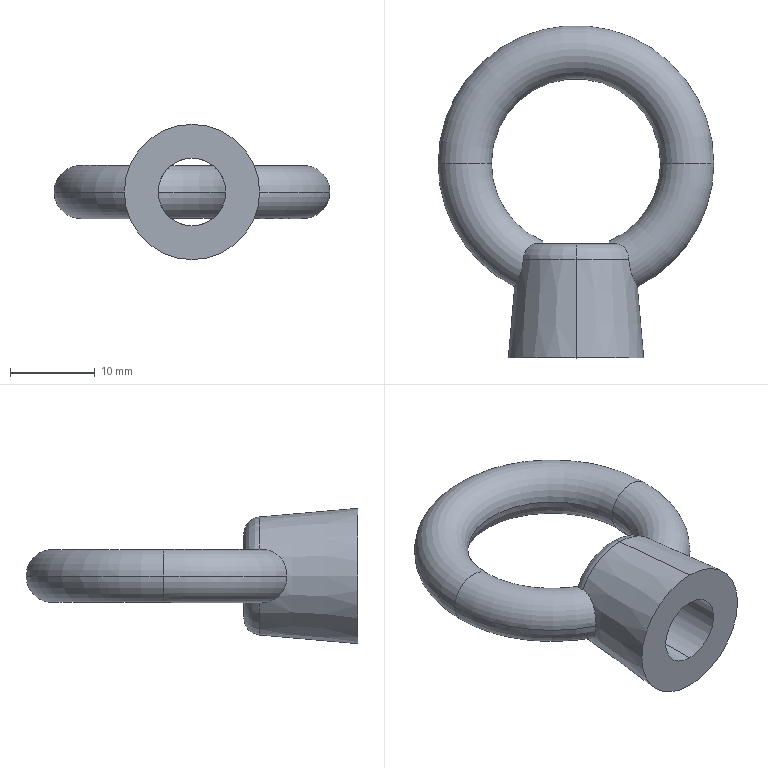Part | STEP file | B-1132-8 | 1 solid | 16 faces | box 32.6 x 39.3 x 16 mm | volume 3782 mm3 | torus 9 | plane 3 | cylinder 2 | cone 2 | commonest cylinder face diameters 8 x2
STEP:
#1=CARTESIAN_POINT('',(16.3,0.,0.));
#2=VERTEX_POINT('',#1);
#3=CARTESIAN_POINT('',(10.,0.,0.));
#4=VERTEX_POINT('',#3);
#5=CARTESIAN_POINT('',(13.15,0.,0.));
#6=DIRECTION('',(0.,1.,0.));
#7=DIRECTION('',(-1.,0.,0.));
#8=AXIS2_PLACEMENT_3D('',#5,#6,#7);
#9=CIRCLE('',#8,3.15);
#10=EDGE_CURVE('',#2,#4,#9,.T.);
#11=ORIENTED_EDGE('',*,*,#10,.F.);
#12=CARTESIAN_POINT('',(7.264,-14.592,0.));
#13=VERTEX_POINT('',#12);
#14=CARTESIAN_POINT('',(0.,0.,0.));
#15=DIRECTION('',(0.,0.,-1.));
#16=DIRECTION('',(-1.,0.,0.));
#17=AXIS2_PLACEMENT_3D('',#14,#15,#16);
#18=CIRCLE('',#17,16.3);
#19=EDGE_CURVE('',#2,#13,#18,.T.);
#20=ORIENTED_EDGE('',*,*,#19,.T.);
#21=CARTESIAN_POINT('',(6.231,-11.326,-3.142));
#22=VERTEX_POINT('',#21);
#23=CARTESIAN_POINT('',(7.264,-14.592,0.));
#24=CARTESIAN_POINT('',(7.264,-14.592,-0.2184));
#25=CARTESIAN_POINT('',(7.253,-14.572,-0.4352));
#26=CARTESIAN_POINT('',(7.207,-14.494,-0.8657));
#27=CARTESIAN_POINT('',(7.173,-14.435,-1.075));
#28=CARTESIAN_POINT('',(7.088,-14.28,-1.474));
#29=CARTESIAN_POINT('',(7.036,-14.183,-1.666));
#30=CARTESIAN_POINT('',(6.922,-13.953,-2.022));
#31=CARTESIAN_POINT('',(6.859,-13.822,-2.184));
#32=CARTESIAN_POINT('',(6.731,-13.524,-2.478));
#33=CARTESIAN_POINT('',(6.665,-13.357,-2.61));
#34=CARTESIAN_POINT('',(6.541,-13.001,-2.828));
#35=CARTESIAN_POINT('',(6.483,-12.81,-2.918));
#36=CARTESIAN_POINT('',(6.38,-12.403,-3.055));
#37=CARTESIAN_POINT('',(6.337,-12.194,-3.101));
#38=CARTESIAN_POINT('',(6.27,-11.765,-3.152));
#39=CARTESIAN_POINT('',(6.246,-11.544,-3.156));
#40=CARTESIAN_POINT('',(6.231,-11.326,-3.142));
#41=B_SPLINE_CURVE_WITH_KNOTS('',3,(#23,#24,#25,#26,#27,#28,#29,#30,#31,#32,#33,#34,#35,#36,#37,#38,#39,#40),.UNSPECIFIED.,.F.,.F.,(4,2,2,2,2,2,2,2,4),(0.007106,0.007756,0.008406,0.009056,0.009706,0.01036,0.01101,0.01166,0.01231),.UNSPECIFIED.);
#42=EDGE_CURVE('',#13,#22,#41,.T.);
#43=ORIENTED_EDGE('',*,*,#42,.T.);
#44=CARTESIAN_POINT('',(4.645,-9.5,-1.814));
#45=VERTEX_POINT('',#44);
#46=CARTESIAN_POINT('',(6.231,-11.326,-3.142));
#47=CARTESIAN_POINT('',(6.223,-11.199,-3.134));
#48=CARTESIAN_POINT('',(6.205,-11.075,-3.119));
#49=CARTESIAN_POINT('',(6.15,-10.834,-3.075));
#50=CARTESIAN_POINT('',(6.113,-10.715,-3.046));
#51=CARTESIAN_POINT('',(6.024,-10.49,-2.971));
#52=CARTESIAN_POINT('',(5.972,-10.385,-2.927));
#53=CARTESIAN_POINT('',(5.855,-10.187,-2.824));
#54=CARTESIAN_POINT('',(5.788,-10.095,-2.765));
#55=CARTESIAN_POINT('',(5.575,-9.848,-2.574));
#56=CARTESIAN_POINT('',(5.411,-9.719,-2.422));
#57=CARTESIAN_POINT('',(5.055,-9.547,-2.112));
#58=CARTESIAN_POINT('',(4.861,-9.5,-1.949));
#59=CARTESIAN_POINT('',(4.645,-9.5,-1.814));
#60=B_SPLINE_CURVE_WITH_KNOTS('',3,(#46,#47,#48,#49,#50,#51,#52,#53,#54,#55,#56,#57,#58,#59),.UNSPECIFIED.,.F.,.F.,(4,2,2,2,2,2,4),(0.,0.0003768,0.0007536,0.00113,0.001507,0.002261,0.003014),.UNSPECIFIED.);
#61=EDGE_CURVE('',#22,#45,#60,.T.);
#62=ORIENTED_EDGE('',*,*,#61,.T.);
#63=CARTESIAN_POINT('',(3.816,-9.5,-1.2));
#64=VERTEX_POINT('',#63);
#65=CARTESIAN_POINT('',(4.645,-9.5,-1.814));
#66=CARTESIAN_POINT('',(4.5,-9.5,-1.723));
#67=CARTESIAN_POINT('',(4.357,-9.5,-1.628));
#68=CARTESIAN_POINT('',(4.08,-9.5,-1.425));
#69=CARTESIAN_POINT('',(3.944,-9.5,-1.316));
#70=CARTESIAN_POINT('',(3.816,-9.5,-1.2));
#71=B_SPLINE_CURVE_WITH_KNOTS('',3,(#65,#66,#67,#68,#69,#70),.UNSPECIFIED.,.F.,.F.,(4,2,4),(0.02444,0.02495,0.02546),.UNSPECIFIED.);
#72=EDGE_CURVE('',#45,#64,#71,.T.);
#73=ORIENTED_EDGE('',*,*,#72,.T.);
#74=CARTESIAN_POINT('',(4.,-9.165,0.));
#75=VERTEX_POINT('',#74);
#76=CARTESIAN_POINT('',(3.816,-9.5,-1.2));
#77=CARTESIAN_POINT('',(3.872,-9.398,-1.021));
#78=CARTESIAN_POINT('',(3.918,-9.314,-0.8311));
#79=CARTESIAN_POINT('',(3.983,-9.196,-0.4221));
#80=CARTESIAN_POINT('',(4.,-9.165,-0.2133));
#81=CARTESIAN_POINT('',(4.,-9.165,0.));
#82=B_SPLINE_CURVE_WITH_KNOTS('',3,(#76,#77,#78,#79,#80,#81),.UNSPECIFIED.,.F.,.F.,(4,2,4),(0.00665,0.007285,0.00792),.UNSPECIFIED.);
#83=EDGE_CURVE('',#64,#75,#82,.T.);
#84=ORIENTED_EDGE('',*,*,#83,.T.);
#85=CARTESIAN_POINT('',(0.,0.,0.));
#86=DIRECTION('',(0.,0.,-1.));
#87=DIRECTION('',(-1.,0.,0.));
#88=AXIS2_PLACEMENT_3D('',#85,#86,#87);
#89=CIRCLE('',#88,10.);
#90=EDGE_CURVE('',#4,#75,#89,.T.);
#91=ORIENTED_EDGE('',*,*,#90,.F.);
#92=EDGE_LOOP('',(#11,#20,#43,#62,#73,#84,#91));
#93=FACE_OUTER_BOUND('',#92,.T.);
#94=CARTESIAN_POINT('',(0.,0.,0.));
#95=DIRECTION('',(0.,0.,-1.));
#96=DIRECTION('',(-1.,0.,0.));
#97=AXIS2_PLACEMENT_3D('',#94,#95,#96);
#98=TOROIDAL_SURFACE('',#97,13.15,3.15);
#99=ADVANCED_FACE('',(#93),#98,.T.);
#100=CARTESIAN_POINT('',(-6.231,-11.326,-3.142));
#101=VERTEX_POINT('',#100);
#102=CARTESIAN_POINT('',(-7.264,-14.592,0.));
#103=VERTEX_POINT('',#102);
#104=CARTESIAN_POINT('',(-6.231,-11.326,-3.142));
#105=CARTESIAN_POINT('',(-6.246,-11.543,-3.156));
#106=CARTESIAN_POINT('',(-6.269,-11.76,-3.152));
#107=CARTESIAN_POINT('',(-6.336,-12.191,-3.101));
#108=CARTESIAN_POINT('',(-6.38,-12.403,-3.055));
#109=CARTESIAN_POINT('',(-6.481,-12.804,-2.92));
#110=CARTESIAN_POINT('',(-6.54,-12.997,-2.831));
#111=CARTESIAN_POINT('',(-6.665,-13.357,-2.61));
#112=CARTESIAN_POINT('',(-6.729,-13.52,-2.482));
#113=CARTESIAN_POINT('',(-6.858,-13.819,-2.188));
#114=CARTESIAN_POINT('',(-6.922,-13.953,-2.022));
#115=CARTESIAN_POINT('',(-7.036,-14.181,-1.668));
#116=CARTESIAN_POINT('',(-7.087,-14.278,-1.478));
#117=CARTESIAN_POINT('',(-7.174,-14.435,-1.075));
#118=CARTESIAN_POINT('',(-7.207,-14.493,-0.8672));
#119=CARTESIAN_POINT('',(-7.252,-14.572,-0.4401));
#120=CARTESIAN_POINT('',(-7.264,-14.592,-0.2184));
#121=CARTESIAN_POINT('',(-7.264,-14.592,0.));
#122=B_SPLINE_CURVE_WITH_KNOTS('',3,(#104,#105,#106,#107,#108,#109,#110,#111,#112,#113,#114,#115,#116,#117,#118,#119,#120,#121),.UNSPECIFIED.,.F.,.F.,(4,2,2,2,2,2,2,2,4),(0.001904,0.002554,0.003205,0.003855,0.004505,0.005155,0.005805,0.006456,0.007106),.UNSPECIFIED.);
#123=EDGE_CURVE('',#101,#103,#122,.T.);
#124=ORIENTED_EDGE('',*,*,#123,.T.);
#125=CARTESIAN_POINT('',(-16.3,0.,0.));
#126=VERTEX_POINT('',#125);
#127=CARTESIAN_POINT('',(0.,0.,0.));
#128=DIRECTION('',(0.,0.,-1.));
#129=DIRECTION('',(-1.,0.,0.));
#130=AXIS2_PLACEMENT_3D('',#127,#128,#129);
#131=CIRCLE('',#130,16.3);
#132=EDGE_CURVE('',#103,#126,#131,.T.);
#133=ORIENTED_EDGE('',*,*,#132,.T.);
#134=CARTESIAN_POINT('',(-10.,0.,0.));
#135=VERTEX_POINT('',#134);
#136=CARTESIAN_POINT('',(-13.15,0.,0.));
#137=DIRECTION('',(0.,-1.,0.));
#138=DIRECTION('',(0.,0.,-1.));
#139=AXIS2_PLACEMENT_3D('',#136,#137,#138);
#140=CIRCLE('',#139,3.15);
#141=EDGE_CURVE('',#126,#135,#140,.T.);
#142=ORIENTED_EDGE('',*,*,#141,.T.);
#143=CARTESIAN_POINT('',(-4.,-9.165,0.));
#144=VERTEX_POINT('',#143);
#145=CARTESIAN_POINT('',(0.,0.,0.));
#146=DIRECTION('',(0.,0.,-1.));
#147=DIRECTION('',(-1.,0.,0.));
#148=AXIS2_PLACEMENT_3D('',#145,#146,#147);
#149=CIRCLE('',#148,10.);
#150=EDGE_CURVE('',#144,#135,#149,.T.);
#151=ORIENTED_EDGE('',*,*,#150,.F.);
#152=CARTESIAN_POINT('',(-3.816,-9.5,-1.2));
#153=VERTEX_POINT('',#152);
#154=CARTESIAN_POINT('',(-4.,-9.165,0.));
#155=CARTESIAN_POINT('',(-4.,-9.165,-0.1064));
#156=CARTESIAN_POINT('',(-3.996,-9.173,-0.2143));
#157=CARTESIAN_POINT('',(-3.979,-9.204,-0.4241));
#158=CARTESIAN_POINT('',(-3.966,-9.226,-0.527));
#159=CARTESIAN_POINT('',(-3.918,-9.314,-0.8302));
#160=CARTESIAN_POINT('',(-3.871,-9.399,-1.023));
#161=CARTESIAN_POINT('',(-3.816,-9.5,-1.2));
#162=B_SPLINE_CURVE_WITH_KNOTS('',3,(#154,#155,#156,#157,#158,#159,#160,#161),.UNSPECIFIED.,.F.,.F.,(4,2,2,4),(0.00792,0.008237,0.008554,0.009188),.UNSPECIFIED.);
#163=EDGE_CURVE('',#144,#153,#162,.T.);
#164=ORIENTED_EDGE('',*,*,#163,.T.);
#165=CARTESIAN_POINT('',(-4.645,-9.5,-1.814));
#166=VERTEX_POINT('',#165);
#167=CARTESIAN_POINT('',(-3.816,-9.5,-1.2));
#168=CARTESIAN_POINT('',(-3.943,-9.5,-1.316));
#169=CARTESIAN_POINT('',(-4.079,-9.5,-1.424));
#170=CARTESIAN_POINT('',(-4.357,-9.5,-1.628));
#171=CARTESIAN_POINT('',(-4.499,-9.5,-1.723));
#172=CARTESIAN_POINT('',(-4.645,-9.5,-1.814));
#173=B_SPLINE_CURVE_WITH_KNOTS('',3,(#167,#168,#169,#170,#171,#172),.UNSPECIFIED.,.F.,.F.,(4,2,4),(0.0236,0.02411,0.02462),.UNSPECIFIED.);
#174=EDGE_CURVE('',#153,#166,#173,.T.);
#175=ORIENTED_EDGE('',*,*,#174,.T.);
#176=CARTESIAN_POINT('',(-4.645,-9.5,-1.814));
#177=CARTESIAN_POINT('',(-4.753,-9.5,-1.881));
#178=CARTESIAN_POINT('',(-4.854,-9.512,-1.955));
#179=CARTESIAN_POINT('',(-5.049,-9.556,-2.108));
#180=CARTESIAN_POINT('',(-5.143,-9.589,-2.188));
#181=CARTESIAN_POINT('',(-5.322,-9.676,-2.344));
#182=CARTESIAN_POINT('',(-5.407,-9.729,-2.42));
#183=CARTESIAN_POINT('',(-5.568,-9.856,-2.567));
#184=CARTESIAN_POINT('',(-5.646,-9.93,-2.637));
#185=CARTESIAN_POINT('',(-5.788,-10.094,-2.765));
#186=CARTESIAN_POINT('',(-5.853,-10.185,-2.823));
#187=CARTESIAN_POINT('',(-5.971,-10.382,-2.926));
#188=CARTESIAN_POINT('',(-6.024,-10.49,-2.971));
#189=CARTESIAN_POINT('',(-6.157,-10.825,-3.082));
#190=CARTESIAN_POINT('',(-6.215,-11.072,-3.126));
#191=CARTESIAN_POINT('',(-6.231,-11.326,-3.142));
#192=B_SPLINE_CURVE_WITH_KNOTS('',3,(#176,#177,#178,#179,#180,#181,#182,#183,#184,#185,#186,#187,#188,#189,#190,#191),.UNSPECIFIED.,.F.,.F.,(4,2,2,2,2,2,2,4),(0.,0.0003768,0.0007535,0.00113,0.001507,0.001884,0.002261,0.003014),.UNSPECIFIED.);
#193=EDGE_CURVE('',#166,#101,#192,.T.);
#194=ORIENTED_EDGE('',*,*,#193,.T.);
#195=EDGE_LOOP('',(#124,#133,#142,#151,#164,#175,#194));
#196=FACE_OUTER_BOUND('',#195,.T.);
#197=CARTESIAN_POINT('',(0.,0.,0.));
#198=DIRECTION('',(0.,0.,-1.));
#199=DIRECTION('',(-1.,0.,0.));
#200=AXIS2_PLACEMENT_3D('',#197,#198,#199);
#201=TOROIDAL_SURFACE('',#200,13.15,3.15);
#202=ADVANCED_FACE('',(#196),#201,.T.);
#203=ORIENTED_EDGE('',*,*,#141,.F.);
#204=CARTESIAN_POINT('',(0.,0.,0.));
#205=DIRECTION('',(0.,0.,-1.));
#206=DIRECTION('',(-1.,0.,0.));
#207=AXIS2_PLACEMENT_3D('',#204,#205,#206);
#208=CIRCLE('',#207,16.3);
#209=EDGE_CURVE('',#126,#2,#208,.T.);
#210=ORIENTED_EDGE('',*,*,#209,.T.);
#211=ORIENTED_EDGE('',*,*,#10,.T.);
#212=CARTESIAN_POINT('',(0.,0.,0.));
#213=DIRECTION('',(0.,0.,-1.));
#214=DIRECTION('',(-1.,0.,0.));
#215=AXIS2_PLACEMENT_3D('',#212,#213,#214);
#216=CIRCLE('',#215,10.);
#217=EDGE_CURVE('',#135,#4,#216,.T.);
#218=ORIENTED_EDGE('',*,*,#217,.F.);
#219=EDGE_LOOP('',(#203,#210,#211,#218));
#220=FACE_OUTER_BOUND('',#219,.T.);
#221=CARTESIAN_POINT('',(0.,0.,0.));
#222=DIRECTION('',(0.,0.,-1.));
#223=DIRECTION('',(-1.,0.,0.));
#224=AXIS2_PLACEMENT_3D('',#221,#222,#223);
#225=TOROIDAL_SURFACE('',#224,13.15,3.15);
#226=ADVANCED_FACE('',(#220),#225,.T.);
#227=CARTESIAN_POINT('',(0.,-11.326,6.979));
#228=VERTEX_POINT('',#227);
#229=CARTESIAN_POINT('',(-6.231,-11.326,3.142));
#230=VERTEX_POINT('',#229);
#231=CARTESIAN_POINT('',(0.,-11.326,0.));
#232=DIRECTION('',(0.,-1.,0.));
#233=DIRECTION('',(0.,0.,1.));
#234=AXIS2_PLACEMENT_3D('',#231,#232,#233);
#235=CIRCLE('',#234,6.979);
#236=EDGE_CURVE('',#228,#230,#235,.T.);
#237=ORIENTED_EDGE('',*,*,#236,.F.);
#238=CARTESIAN_POINT('',(0.,-9.5,4.986));
#239=VERTEX_POINT('',#238);
#240=CARTESIAN_POINT('',(0.,-11.5,4.986));
#241=DIRECTION('',(-1.,0.,0.));
#242=DIRECTION('',(0.,0.,1.));
#243=AXIS2_PLACEMENT_3D('',#240,#241,#242);
#244=CIRCLE('',#243,2.);
#245=EDGE_CURVE('',#228,#239,#244,.T.);
#246=ORIENTED_EDGE('',*,*,#245,.T.);
#247=CARTESIAN_POINT('',(-4.645,-9.5,1.814));
#248=VERTEX_POINT('',#247);
#249=CARTESIAN_POINT('',(0.,-9.5,0.));
#250=DIRECTION('',(0.,1.,0.));
#251=DIRECTION('',(0.,0.,1.));
#252=AXIS2_PLACEMENT_3D('',#249,#250,#251);
#253=CIRCLE('',#252,4.986);
#254=EDGE_CURVE('',#248,#239,#253,.T.);
#255=ORIENTED_EDGE('',*,*,#254,.F.);
#256=CARTESIAN_POINT('',(-6.231,-11.326,3.142));
#257=CARTESIAN_POINT('',(-6.223,-11.199,3.134));
#258=CARTESIAN_POINT('',(-6.205,-11.075,3.119));
#259=CARTESIAN_POINT('',(-6.15,-10.834,3.075));
#260=CARTESIAN_POINT('',(-6.113,-10.715,3.046));
#261=CARTESIAN_POINT('',(-6.024,-10.49,2.971));
#262=CARTESIAN_POINT('',(-5.972,-10.385,2.927));
#263=CARTESIAN_POINT('',(-5.855,-10.187,2.824));
#264=CARTESIAN_POINT('',(-5.788,-10.095,2.765));
#265=CARTESIAN_POINT('',(-5.575,-9.848,2.574));
#266=CARTESIAN_POINT('',(-5.411,-9.719,2.422));
#267=CARTESIAN_POINT('',(-5.055,-9.547,2.112));
#268=CARTESIAN_POINT('',(-4.861,-9.5,1.949));
#269=CARTESIAN_POINT('',(-4.645,-9.5,1.814));
#270=B_SPLINE_CURVE_WITH_KNOTS('',3,(#256,#257,#258,#259,#260,#261,#262,#263,#264,#265,#266,#267,#268,#269),.UNSPECIFIED.,.F.,.F.,(4,2,2,2,2,2,4),(0.,0.0003768,0.0007536,0.00113,0.001507,0.002261,0.003014),.UNSPECIFIED.);
#271=EDGE_CURVE('',#230,#248,#270,.T.);
#272=ORIENTED_EDGE('',*,*,#271,.F.);
#273=EDGE_LOOP('',(#237,#246,#255,#272));
#274=FACE_OUTER_BOUND('',#273,.T.);
#275=CARTESIAN_POINT('',(0.,-11.5,0.));
#276=DIRECTION('',(0.,1.,0.));
#277=DIRECTION('',(0.,0.,1.));
#278=AXIS2_PLACEMENT_3D('',#275,#276,#277);
#279=TOROIDAL_SURFACE('',#278,4.986,2.);
#280=ADVANCED_FACE('',(#274),#279,.T.);
#281=CARTESIAN_POINT('',(-3.816,-9.5,1.2));
#282=VERTEX_POINT('',#281);
#283=CARTESIAN_POINT('',(0.,-9.5,4.));
#284=VERTEX_POINT('',#283);
#285=CARTESIAN_POINT('',(0.,-9.5,0.));
#286=DIRECTION('',(0.,1.,0.));
#287=DIRECTION('',(0.,0.,1.));
#288=AXIS2_PLACEMENT_3D('',#285,#286,#287);
#289=CIRCLE('',#288,4.);
#290=EDGE_CURVE('',#282,#284,#289,.T.);
#291=ORIENTED_EDGE('',*,*,#290,.T.);
#292=CARTESIAN_POINT('',(0.,-23.,4.));
#293=VERTEX_POINT('',#292);
#294=CARTESIAN_POINT('',(0.,-5.,4.));
#295=DIRECTION('',(0.,-1.,0.));
#296=VECTOR('',#295,1000.);
#297=LINE('',#294,#296);
#298=EDGE_CURVE('',#284,#293,#297,.T.);
#299=ORIENTED_EDGE('',*,*,#298,.T.);
#300=CARTESIAN_POINT('',(0.,-23.,-4.));
#301=VERTEX_POINT('',#300);
#302=CARTESIAN_POINT('',(0.,-23.,0.));
#303=DIRECTION('',(0.,-1.,0.));
#304=DIRECTION('',(0.,0.,-1.));
#305=AXIS2_PLACEMENT_3D('',#302,#303,#304);
#306=CIRCLE('',#305,4.);
#307=EDGE_CURVE('',#293,#301,#306,.T.);
#308=ORIENTED_EDGE('',*,*,#307,.T.);
#309=CARTESIAN_POINT('',(0.,-9.5,-4.));
#310=VERTEX_POINT('',#309);
#311=CARTESIAN_POINT('',(0.,-5.,-4.));
#312=DIRECTION('',(0.,-1.,0.));
#313=VECTOR('',#312,1000.);
#314=LINE('',#311,#313);
#315=EDGE_CURVE('',#310,#301,#314,.T.);
#316=ORIENTED_EDGE('',*,*,#315,.F.);
#317=CARTESIAN_POINT('',(0.,-9.5,0.));
#318=DIRECTION('',(0.,1.,0.));
#319=DIRECTION('',(0.,0.,1.));
#320=AXIS2_PLACEMENT_3D('',#317,#318,#319);
#321=CIRCLE('',#320,4.);
#322=EDGE_CURVE('',#310,#153,#321,.T.);
#323=ORIENTED_EDGE('',*,*,#322,.T.);
#324=ORIENTED_EDGE('',*,*,#163,.F.);
#325=CARTESIAN_POINT('',(-3.816,-9.5,1.2));
#326=CARTESIAN_POINT('',(-3.872,-9.398,1.021));
#327=CARTESIAN_POINT('',(-3.918,-9.314,0.8311));
#328=CARTESIAN_POINT('',(-3.983,-9.196,0.4221));
#329=CARTESIAN_POINT('',(-4.,-9.165,0.2133));
#330=CARTESIAN_POINT('',(-4.,-9.165,0.));
#331=B_SPLINE_CURVE_WITH_KNOTS('',3,(#325,#326,#327,#328,#329,#330),.UNSPECIFIED.,.F.,.F.,(4,2,4),(0.00665,0.007285,0.00792),.UNSPECIFIED.);
#332=EDGE_CURVE('',#282,#144,#331,.T.);
#333=ORIENTED_EDGE('',*,*,#332,.F.);
#334=EDGE_LOOP('',(#291,#299,#308,#316,#323,#324,#333));
#335=FACE_OUTER_BOUND('',#334,.T.);
#336=CARTESIAN_POINT('',(0.,-5.,0.));
#337=DIRECTION('',(0.,-1.,0.));
#338=DIRECTION('',(0.,0.,-1.));
#339=AXIS2_PLACEMENT_3D('',#336,#337,#338);
#340=CYLINDRICAL_SURFACE('',#339,4.);
#341=ADVANCED_FACE('',(#335),#340,.F.);
#342=ORIENTED_EDGE('',*,*,#209,.F.);
#343=CARTESIAN_POINT('',(-13.15,0.,0.));
#344=DIRECTION('',(0.,-1.,0.));
#345=DIRECTION('',(0.,0.,-1.));
#346=AXIS2_PLACEMENT_3D('',#343,#344,#345);
#347=CIRCLE('',#346,3.15);
#348=EDGE_CURVE('',#135,#126,#347,.T.);
#349=ORIENTED_EDGE('',*,*,#348,.F.);
#350=ORIENTED_EDGE('',*,*,#217,.T.);
#351=CARTESIAN_POINT('',(13.15,0.,0.));
#352=DIRECTION('',(0.,1.,0.));
#353=DIRECTION('',(-1.,0.,0.));
#354=AXIS2_PLACEMENT_3D('',#351,#352,#353);
#355=CIRCLE('',#354,3.15);
#356=EDGE_CURVE('',#4,#2,#355,.T.);
#357=ORIENTED_EDGE('',*,*,#356,.T.);
#358=EDGE_LOOP('',(#342,#349,#350,#357));
#359=FACE_OUTER_BOUND('',#358,.T.);
#360=CARTESIAN_POINT('',(0.,0.,0.));
#361=DIRECTION('',(0.,0.,-1.));
#362=DIRECTION('',(-1.,0.,0.));
#363=AXIS2_PLACEMENT_3D('',#360,#361,#362);
#364=TOROIDAL_SURFACE('',#363,13.15,3.15);
#365=ADVANCED_FACE('',(#359),#364,.T.);
#366=ORIENTED_EDGE('',*,*,#132,.F.);
#367=CARTESIAN_POINT('',(-7.264,-14.592,0.));
#368=CARTESIAN_POINT('',(-7.264,-14.592,0.2184));
#369=CARTESIAN_POINT('',(-7.253,-14.572,0.4352));
#370=CARTESIAN_POINT('',(-7.207,-14.494,0.8657));
#371=CARTESIAN_POINT('',(-7.173,-14.435,1.075));
#372=CARTESIAN_POINT('',(-7.088,-14.28,1.474));
#373=CARTESIAN_POINT('',(-7.036,-14.183,1.666));
#374=CARTESIAN_POINT('',(-6.922,-13.953,2.022));
#375=CARTESIAN_POINT('',(-6.859,-13.822,2.184));
#376=CARTESIAN_POINT('',(-6.731,-13.524,2.478));
#377=CARTESIAN_POINT('',(-6.665,-13.357,2.61));
#378=CARTESIAN_POINT('',(-6.541,-13.001,2.828));
#379=CARTESIAN_POINT('',(-6.483,-12.81,2.918));
#380=CARTESIAN_POINT('',(-6.38,-12.403,3.055));
#381=CARTESIAN_POINT('',(-6.337,-12.194,3.101));
#382=CARTESIAN_POINT('',(-6.27,-11.765,3.152));
#383=CARTESIAN_POINT('',(-6.246,-11.544,3.156));
#384=CARTESIAN_POINT('',(-6.231,-11.326,3.142));
#385=B_SPLINE_CURVE_WITH_KNOTS('',3,(#367,#368,#369,#370,#371,#372,#373,#374,#375,#376,#377,#378,#379,#380,#381,#382,#383,#384),.UNSPECIFIED.,.F.,.F.,(4,2,2,2,2,2,2,2,4),(0.007106,0.007756,0.008406,0.009056,0.009706,0.01036,0.01101,0.01166,0.01231),.UNSPECIFIED.);
#386=EDGE_CURVE('',#103,#230,#385,.T.);
#387=ORIENTED_EDGE('',*,*,#386,.T.);
#388=ORIENTED_EDGE('',*,*,#271,.T.);
#389=CARTESIAN_POINT('',(-4.645,-9.5,1.814));
#390=CARTESIAN_POINT('',(-4.5,-9.5,1.723));
#391=CARTESIAN_POINT('',(-4.357,-9.5,1.628));
#392=CARTESIAN_POINT('',(-4.08,-9.5,1.425));
#393=CARTESIAN_POINT('',(-3.944,-9.5,1.316));
#394=CARTESIAN_POINT('',(-3.816,-9.5,1.2));
#395=B_SPLINE_CURVE_WITH_KNOTS('',3,(#389,#390,#391,#392,#393,#394),.UNSPECIFIED.,.F.,.F.,(4,2,4),(0.01978,0.02029,0.0208),.UNSPECIFIED.);
#396=EDGE_CURVE('',#248,#282,#395,.T.);
#397=ORIENTED_EDGE('',*,*,#396,.T.);
#398=ORIENTED_EDGE('',*,*,#332,.T.);
#399=ORIENTED_EDGE('',*,*,#150,.T.);
#400=ORIENTED_EDGE('',*,*,#348,.T.);
#401=EDGE_LOOP('',(#366,#387,#388,#397,#398,#399,#400));
#402=FACE_OUTER_BOUND('',#401,.T.);
#403=CARTESIAN_POINT('',(0.,0.,0.));
#404=DIRECTION('',(0.,0.,-1.));
#405=DIRECTION('',(-1.,0.,0.));
#406=AXIS2_PLACEMENT_3D('',#403,#404,#405);
#407=TOROIDAL_SURFACE('',#406,13.15,3.15);
#408=ADVANCED_FACE('',(#402),#407,.T.);
#409=CARTESIAN_POINT('',(6.231,-11.326,3.142));
#410=VERTEX_POINT('',#409);
#411=CARTESIAN_POINT('',(0.,-11.326,0.));
#412=DIRECTION('',(0.,-1.,0.));
#413=DIRECTION('',(0.,0.,1.));
#414=AXIS2_PLACEMENT_3D('',#411,#412,#413);
#415=CIRCLE('',#414,6.979);
#416=EDGE_CURVE('',#410,#228,#415,.T.);
#417=ORIENTED_EDGE('',*,*,#416,.T.);
#418=CARTESIAN_POINT('',(0.,-23.,8.));
#419=VERTEX_POINT('',#418);
#420=CARTESIAN_POINT('',(0.,-9.5,6.819));
#421=DIRECTION('',(0.,-0.9962,0.08716));
#422=VECTOR('',#421,1000.);
#423=LINE('',#420,#422);
#424=EDGE_CURVE('',#228,#419,#423,.T.);
#425=ORIENTED_EDGE('',*,*,#424,.T.);
#426=CARTESIAN_POINT('',(0.,-23.,-8.));
#427=VERTEX_POINT('',#426);
#428=CARTESIAN_POINT('',(0.,-23.,0.));
#429=DIRECTION('',(0.,1.,0.));
#430=DIRECTION('',(0.,0.,1.));
#431=AXIS2_PLACEMENT_3D('',#428,#429,#430);
#432=CIRCLE('',#431,8.);
#433=EDGE_CURVE('',#419,#427,#432,.T.);
#434=ORIENTED_EDGE('',*,*,#433,.T.);
#435=CARTESIAN_POINT('',(0.,-11.326,-6.979));
#436=VERTEX_POINT('',#435);
#437=CARTESIAN_POINT('',(0.,-9.5,-6.819));
#438=DIRECTION('',(0.,-0.9962,-0.08716));
#439=VECTOR('',#438,1000.);
#440=LINE('',#437,#439);
#441=EDGE_CURVE('',#436,#427,#440,.T.);
#442=ORIENTED_EDGE('',*,*,#441,.F.);
#443=CARTESIAN_POINT('',(0.,-11.326,0.));
#444=DIRECTION('',(0.,-1.,0.));
#445=DIRECTION('',(0.,0.,1.));
#446=AXIS2_PLACEMENT_3D('',#443,#444,#445);
#447=CIRCLE('',#446,6.979);
#448=EDGE_CURVE('',#436,#22,#447,.T.);
#449=ORIENTED_EDGE('',*,*,#448,.T.);
#450=ORIENTED_EDGE('',*,*,#42,.F.);
#451=CARTESIAN_POINT('',(6.231,-11.326,3.142));
#452=CARTESIAN_POINT('',(6.246,-11.543,3.156));
#453=CARTESIAN_POINT('',(6.269,-11.76,3.152));
#454=CARTESIAN_POINT('',(6.336,-12.191,3.101));
#455=CARTESIAN_POINT('',(6.38,-12.403,3.055));
#456=CARTESIAN_POINT('',(6.481,-12.804,2.92));
#457=CARTESIAN_POINT('',(6.54,-12.997,2.831));
#458=CARTESIAN_POINT('',(6.665,-13.357,2.61));
#459=CARTESIAN_POINT('',(6.729,-13.52,2.482));
#460=CARTESIAN_POINT('',(6.858,-13.819,2.188));
#461=CARTESIAN_POINT('',(6.922,-13.953,2.022));
#462=CARTESIAN_POINT('',(7.036,-14.181,1.668));
#463=CARTESIAN_POINT('',(7.087,-14.278,1.478));
#464=CARTESIAN_POINT('',(7.174,-14.435,1.075));
#465=CARTESIAN_POINT('',(7.207,-14.493,0.8672));
#466=CARTESIAN_POINT('',(7.252,-14.572,0.4401));
#467=CARTESIAN_POINT('',(7.264,-14.592,0.2184));
#468=CARTESIAN_POINT('',(7.264,-14.592,0.));
#469=B_SPLINE_CURVE_WITH_KNOTS('',3,(#451,#452,#453,#454,#455,#456,#457,#458,#459,#460,#461,#462,#463,#464,#465,#466,#467,#468),.UNSPECIFIED.,.F.,.F.,(4,2,2,2,2,2,2,2,4),(0.001904,0.002554,0.003205,0.003855,0.004505,0.005155,0.005805,0.006456,0.007106),.UNSPECIFIED.);
#470=EDGE_CURVE('',#410,#13,#469,.T.);
#471=ORIENTED_EDGE('',*,*,#470,.F.);
#472=EDGE_LOOP('',(#417,#425,#434,#442,#449,#450,#471));
#473=FACE_OUTER_BOUND('',#472,.T.);
#474=CARTESIAN_POINT('',(0.,-9.5,0.));
#475=DIRECTION('',(0.,-1.,0.));
#476=DIRECTION('',(0.,0.,-1.));
#477=AXIS2_PLACEMENT_3D('',#474,#475,#476);
#478=CONICAL_SURFACE('',#477,6.819,0.08727);
#479=ADVANCED_FACE('',(#473),#478,.T.);
#480=ORIENTED_EDGE('',*,*,#72,.F.);
#481=CARTESIAN_POINT('',(0.,-9.5,0.));
#482=DIRECTION('',(0.,1.,0.));
#483=DIRECTION('',(0.,0.,1.));
#484=AXIS2_PLACEMENT_3D('',#481,#482,#483);
#485=CIRCLE('',#484,4.986);
#486=EDGE_CURVE('',#45,#166,#485,.T.);
#487=ORIENTED_EDGE('',*,*,#486,.T.);
#488=ORIENTED_EDGE('',*,*,#174,.F.);
#489=ORIENTED_EDGE('',*,*,#322,.F.);
#490=CARTESIAN_POINT('',(0.,-9.5,0.));
#491=DIRECTION('',(0.,1.,0.));
#492=DIRECTION('',(0.,0.,1.));
#493=AXIS2_PLACEMENT_3D('',#490,#491,#492);
#494=CIRCLE('',#493,4.);
#495=EDGE_CURVE('',#64,#310,#494,.T.);
#496=ORIENTED_EDGE('',*,*,#495,.F.);
#497=EDGE_LOOP('',(#480,#487,#488,#489,#496));
#498=FACE_OUTER_BOUND('',#497,.T.);
#499=CARTESIAN_POINT('',(-6.819,-9.5,0.));
#500=DIRECTION('',(0.,1.,0.));
#501=DIRECTION('',(0.,0.,1.));
#502=AXIS2_PLACEMENT_3D('',#499,#500,#501);
#503=PLANE('',#502);
#504=ADVANCED_FACE('',(#498),#503,.T.);
#505=ORIENTED_EDGE('',*,*,#424,.F.);
#506=ORIENTED_EDGE('',*,*,#236,.T.);
#507=ORIENTED_EDGE('',*,*,#386,.F.);
#508=ORIENTED_EDGE('',*,*,#123,.F.);
#509=CARTESIAN_POINT('',(0.,-11.326,0.));
#510=DIRECTION('',(0.,-1.,0.));
#511=DIRECTION('',(0.,0.,1.));
#512=AXIS2_PLACEMENT_3D('',#509,#510,#511);
#513=CIRCLE('',#512,6.979);
#514=EDGE_CURVE('',#101,#436,#513,.T.);
#515=ORIENTED_EDGE('',*,*,#514,.T.);
#516=ORIENTED_EDGE('',*,*,#441,.T.);
#517=CARTESIAN_POINT('',(0.,-23.,0.));
#518=DIRECTION('',(0.,1.,0.));
#519=DIRECTION('',(0.,0.,1.));
#520=AXIS2_PLACEMENT_3D('',#517,#518,#519);
#521=CIRCLE('',#520,8.);
#522=EDGE_CURVE('',#427,#419,#521,.T.);
#523=ORIENTED_EDGE('',*,*,#522,.T.);
#524=EDGE_LOOP('',(#505,#506,#507,#508,#515,#516,#523));
#525=FACE_OUTER_BOUND('',#524,.T.);
#526=CARTESIAN_POINT('',(0.,-9.5,0.));
#527=DIRECTION('',(0.,-1.,0.));
#528=DIRECTION('',(0.,0.,-1.));
#529=AXIS2_PLACEMENT_3D('',#526,#527,#528);
#530=CONICAL_SURFACE('',#529,6.819,0.08727);
#531=ADVANCED_FACE('',(#525),#530,.T.);
#532=ORIENTED_EDGE('',*,*,#396,.F.);
#533=ORIENTED_EDGE('',*,*,#254,.T.);
#534=CARTESIAN_POINT('',(4.645,-9.5,1.814));
#535=VERTEX_POINT('',#534);
#536=CARTESIAN_POINT('',(0.,-9.5,0.));
#537=DIRECTION('',(0.,1.,0.));
#538=DIRECTION('',(0.,0.,1.));
#539=AXIS2_PLACEMENT_3D('',#536,#537,#538);
#540=CIRCLE('',#539,4.986);
#541=EDGE_CURVE('',#239,#535,#540,.T.);
#542=ORIENTED_EDGE('',*,*,#541,.T.);
#543=CARTESIAN_POINT('',(3.816,-9.5,1.2));
#544=VERTEX_POINT('',#543);
#545=CARTESIAN_POINT('',(3.816,-9.5,1.2));
#546=CARTESIAN_POINT('',(3.943,-9.5,1.316));
#547=CARTESIAN_POINT('',(4.079,-9.5,1.424));
#548=CARTESIAN_POINT('',(4.357,-9.5,1.628));
#549=CARTESIAN_POINT('',(4.499,-9.5,1.723));
#550=CARTESIAN_POINT('',(4.645,-9.5,1.814));
#551=B_SPLINE_CURVE_WITH_KNOTS('',3,(#545,#546,#547,#548,#549,#550),.UNSPECIFIED.,.F.,.F.,(4,2,4),(0.002615,0.003126,0.003637),.UNSPECIFIED.);
#552=EDGE_CURVE('',#544,#535,#551,.T.);
#553=ORIENTED_EDGE('',*,*,#552,.F.);
#554=CARTESIAN_POINT('',(0.,-9.5,0.));
#555=DIRECTION('',(0.,1.,0.));
#556=DIRECTION('',(0.,0.,1.));
#557=AXIS2_PLACEMENT_3D('',#554,#555,#556);
#558=CIRCLE('',#557,4.);
#559=EDGE_CURVE('',#284,#544,#558,.T.);
#560=ORIENTED_EDGE('',*,*,#559,.F.);
#561=ORIENTED_EDGE('',*,*,#290,.F.);
#562=EDGE_LOOP('',(#532,#533,#542,#553,#560,#561));
#563=FACE_OUTER_BOUND('',#562,.T.);
#564=CARTESIAN_POINT('',(-6.819,-9.5,0.));
#565=DIRECTION('',(0.,1.,0.));
#566=DIRECTION('',(0.,0.,1.));
#567=AXIS2_PLACEMENT_3D('',#564,#565,#566);
#568=PLANE('',#567);
#569=ADVANCED_FACE('',(#563),#568,.T.);
#570=CARTESIAN_POINT('',(0.,-23.,0.));
#571=DIRECTION('',(0.,-1.,0.));
#572=DIRECTION('',(0.,0.,-1.));
#573=AXIS2_PLACEMENT_3D('',#570,#571,#572);
#574=CIRCLE('',#573,4.);
#575=EDGE_CURVE('',#301,#293,#574,.T.);
#576=ORIENTED_EDGE('',*,*,#575,.F.);
#577=ORIENTED_EDGE('',*,*,#307,.F.);
#578=EDGE_LOOP('',(#576,#577));
#579=FACE_BOUND('',#578,.T.);
#580=ORIENTED_EDGE('',*,*,#522,.F.);
#581=ORIENTED_EDGE('',*,*,#433,.F.);
#582=EDGE_LOOP('',(#580,#581));
#583=FACE_OUTER_BOUND('',#582,.T.);
#584=CARTESIAN_POINT('',(-8.,-23.,0.));
#585=DIRECTION('',(0.,-1.,0.));
#586=DIRECTION('',(0.,0.,-1.));
#587=AXIS2_PLACEMENT_3D('',#584,#585,#586);
#588=PLANE('',#587);
#589=ADVANCED_FACE('',(#579,#583),#588,.T.);
#590=ORIENTED_EDGE('',*,*,#19,.F.);
#591=ORIENTED_EDGE('',*,*,#356,.F.);
#592=ORIENTED_EDGE('',*,*,#90,.T.);
#593=CARTESIAN_POINT('',(4.,-9.165,0.));
#594=CARTESIAN_POINT('',(4.,-9.165,0.1064));
#595=CARTESIAN_POINT('',(3.996,-9.173,0.2143));
#596=CARTESIAN_POINT('',(3.979,-9.204,0.4241));
#597=CARTESIAN_POINT('',(3.966,-9.226,0.527));
#598=CARTESIAN_POINT('',(3.918,-9.314,0.8302));
#599=CARTESIAN_POINT('',(3.871,-9.399,1.023));
#600=CARTESIAN_POINT('',(3.816,-9.5,1.2));
#601=B_SPLINE_CURVE_WITH_KNOTS('',3,(#593,#594,#595,#596,#597,#598,#599,#600),.UNSPECIFIED.,.F.,.F.,(4,2,2,4),(0.00792,0.008237,0.008554,0.009188),.UNSPECIFIED.);
#602=EDGE_CURVE('',#75,#544,#601,.T.);
#603=ORIENTED_EDGE('',*,*,#602,.T.);
#604=ORIENTED_EDGE('',*,*,#552,.T.);
#605=CARTESIAN_POINT('',(4.645,-9.5,1.814));
#606=CARTESIAN_POINT('',(4.753,-9.5,1.881));
#607=CARTESIAN_POINT('',(4.854,-9.512,1.955));
#608=CARTESIAN_POINT('',(5.049,-9.556,2.108));
#609=CARTESIAN_POINT('',(5.143,-9.589,2.188));
#610=CARTESIAN_POINT('',(5.322,-9.676,2.344));
#611=CARTESIAN_POINT('',(5.407,-9.729,2.42));
#612=CARTESIAN_POINT('',(5.568,-9.856,2.567));
#613=CARTESIAN_POINT('',(5.646,-9.93,2.637));
#614=CARTESIAN_POINT('',(5.788,-10.094,2.765));
#615=CARTESIAN_POINT('',(5.853,-10.185,2.823));
#616=CARTESIAN_POINT('',(5.971,-10.382,2.926));
#617=CARTESIAN_POINT('',(6.024,-10.49,2.971));
#618=CARTESIAN_POINT('',(6.157,-10.825,3.082));
#619=CARTESIAN_POINT('',(6.215,-11.072,3.126));
#620=CARTESIAN_POINT('',(6.231,-11.326,3.142));
#621=B_SPLINE_CURVE_WITH_KNOTS('',3,(#605,#606,#607,#608,#609,#610,#611,#612,#613,#614,#615,#616,#617,#618,#619,#620),.UNSPECIFIED.,.F.,.F.,(4,2,2,2,2,2,2,4),(0.,0.0003768,0.0007535,0.00113,0.001507,0.001884,0.002261,0.003014),.UNSPECIFIED.);
#622=EDGE_CURVE('',#535,#410,#621,.T.);
#623=ORIENTED_EDGE('',*,*,#622,.T.);
#624=ORIENTED_EDGE('',*,*,#470,.T.);
#625=EDGE_LOOP('',(#590,#591,#592,#603,#604,#623,#624));
#626=FACE_OUTER_BOUND('',#625,.T.);
#627=CARTESIAN_POINT('',(0.,0.,0.));
#628=DIRECTION('',(0.,0.,-1.));
#629=DIRECTION('',(-1.,0.,0.));
#630=AXIS2_PLACEMENT_3D('',#627,#628,#629);
#631=TOROIDAL_SURFACE('',#630,13.15,3.15);
#632=ADVANCED_FACE('',(#626),#631,.T.);
#633=ORIENTED_EDGE('',*,*,#298,.F.);
#634=ORIENTED_EDGE('',*,*,#559,.T.);
#635=ORIENTED_EDGE('',*,*,#602,.F.);
#636=ORIENTED_EDGE('',*,*,#83,.F.);
#637=ORIENTED_EDGE('',*,*,#495,.T.);
#638=ORIENTED_EDGE('',*,*,#315,.T.);
#639=ORIENTED_EDGE('',*,*,#575,.T.);
#640=EDGE_LOOP('',(#633,#634,#635,#636,#637,#638,#639));
#641=FACE_OUTER_BOUND('',#640,.T.);
#642=CARTESIAN_POINT('',(0.,-5.,0.));
#643=DIRECTION('',(0.,-1.,0.));
#644=DIRECTION('',(0.,0.,-1.));
#645=AXIS2_PLACEMENT_3D('',#642,#643,#644);
#646=CYLINDRICAL_SURFACE('',#645,4.);
#647=ADVANCED_FACE('',(#641),#646,.F.);
#648=ORIENTED_EDGE('',*,*,#61,.F.);
#649=ORIENTED_EDGE('',*,*,#448,.F.);
#650=ORIENTED_EDGE('',*,*,#514,.F.);
#651=ORIENTED_EDGE('',*,*,#193,.F.);
#652=ORIENTED_EDGE('',*,*,#486,.F.);
#653=EDGE_LOOP('',(#648,#649,#650,#651,#652));
#654=FACE_OUTER_BOUND('',#653,.T.);
#655=CARTESIAN_POINT('',(0.,-11.5,0.));
#656=DIRECTION('',(0.,1.,0.));
#657=DIRECTION('',(0.,0.,1.));
#658=AXIS2_PLACEMENT_3D('',#655,#656,#657);
#659=TOROIDAL_SURFACE('',#658,4.986,2.);
#660=ADVANCED_FACE('',(#654),#659,.T.);
#661=ORIENTED_EDGE('',*,*,#245,.F.);
#662=ORIENTED_EDGE('',*,*,#416,.F.);
#663=ORIENTED_EDGE('',*,*,#622,.F.);
#664=ORIENTED_EDGE('',*,*,#541,.F.);
#665=EDGE_LOOP('',(#661,#662,#663,#664));
#666=FACE_OUTER_BOUND('',#665,.T.);
#667=CARTESIAN_POINT('',(0.,-11.5,0.));
#668=DIRECTION('',(0.,1.,0.));
#669=DIRECTION('',(0.,0.,1.));
#670=AXIS2_PLACEMENT_3D('',#667,#668,#669);
#671=TOROIDAL_SURFACE('',#670,4.986,2.);
#672=ADVANCED_FACE('',(#666),#671,.T.);
#673=CLOSED_SHELL('',(#99,#202,#226,#280,#341,#365,#408,#479,#504,#531,#569,#589,#632,#647,#660,#672));
#674=MANIFOLD_SOLID_BREP('',#673);
#675=CARTESIAN_POINT('',(0.,0.,0.));
#676=DIRECTION('',(0.,0.,1.));
#677=DIRECTION('',(1.,0.,0.));
#678=AXIS2_PLACEMENT_3D('',#675,#676,#677);
#679=(LENGTH_UNIT()NAMED_UNIT(*)SI_UNIT(.MILLI.,.METRE.));
#680=UNCERTAINTY_MEASURE_WITH_UNIT(LENGTH_MEASURE(0.00001),#679,'','');
#681=(NAMED_UNIT(*)PLANE_ANGLE_UNIT()SI_UNIT($,.RADIAN.));
#682=(NAMED_UNIT(*)SI_UNIT($,.STERADIAN.)SOLID_ANGLE_UNIT());
#683=(GEOMETRIC_REPRESENTATION_CONTEXT(3)GLOBAL_UNCERTAINTY_ASSIGNED_CONTEXT((#680))GLOBAL_UNIT_ASSIGNED_CONTEXT((#679,#681,#682))REPRESENTATION_CONTEXT('',''));
#684=ADVANCED_BREP_SHAPE_REPRESENTATION('',(#674,#678),#683);